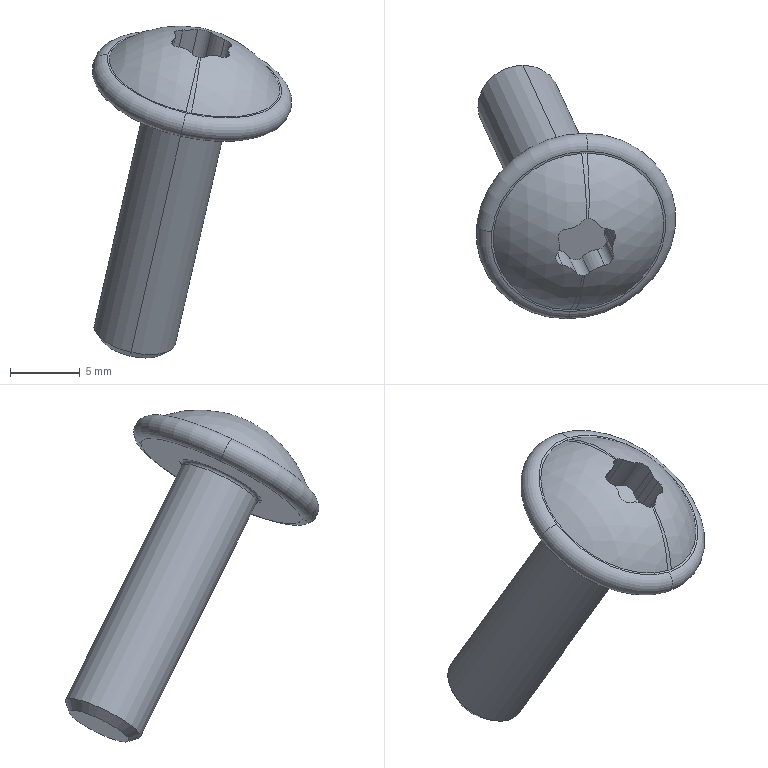Part | SolidWorks | features BaseBody 1 | 1 solid | 32 faces | box 14.289 x 18.177 x 23.78 mm | volume 994.304 mm3 | cylinder 17 | torus 5 | sphere 4 | plane 4 | cone 2 | commonest cylinder face diameters 1.32 x6 3.14 x4 2.34 x3 1.26 x2 6 x2
STEP:
#1=CARTESIAN_POINT('',(1919.161,-253.575,949.426));
#2=VERTEX_POINT('',#1);
#3=CARTESIAN_POINT('',(1919.214,-254.009,949.147));
#4=VERTEX_POINT('',#3);
#5=CARTESIAN_POINT('',(1919.161,-253.575,949.426));
#6=CARTESIAN_POINT('',(1919.144,-253.731,949.352));
#7=CARTESIAN_POINT('',(1919.162,-253.881,949.256));
#8=CARTESIAN_POINT('',(1919.214,-254.009,949.147));
#9=B_SPLINE_CURVE_WITH_KNOTS('',3,(#5,#6,#7,#8),.UNSPECIFIED.,.F.,.F.,(4,4),(0.000521,0.001041),.UNSPECIFIED.);
#10=EDGE_CURVE('',#2,#4,#9,.T.);
#11=ORIENTED_EDGE('',*,*,#10,.F.);
#12=CARTESIAN_POINT('',(1918.622,-252.41,947.083));
#13=VERTEX_POINT('',#12);
#14=CARTESIAN_POINT('',(1919.185,-253.627,949.532));
#15=DIRECTION('',(-0.2015,0.436,-0.8771));
#16=VECTOR('',#15,1000.);
#17=LINE('',#14,#16);
#18=EDGE_CURVE('',#2,#13,#17,.T.);
#19=ORIENTED_EDGE('',*,*,#18,.T.);
#20=CARTESIAN_POINT('',(1918.684,-252.864,946.843));
#21=VERTEX_POINT('',#20);
#22=CARTESIAN_POINT('',(1919.763,-252.41,946.821));
#23=DIRECTION('',(-0.2015,0.436,-0.8771));
#24=DIRECTION('',(-0.9216,-0.3877,0.01896));
#25=AXIS2_PLACEMENT_3D('',#22,#23,#24);
#26=CIRCLE('',#25,1.17);
#27=EDGE_CURVE('',#21,#13,#26,.T.);
#28=ORIENTED_EDGE('',*,*,#27,.F.);
#29=CARTESIAN_POINT('',(1918.684,-252.864,946.843));
#30=DIRECTION('',(0.2015,-0.436,0.8771));
#31=VECTOR('',#30,1000.);
#32=LINE('',#29,#31);
#33=EDGE_CURVE('',#21,#4,#32,.T.);
#34=ORIENTED_EDGE('',*,*,#33,.T.);
#35=EDGE_LOOP('',(#11,#19,#28,#34));
#36=FACE_OUTER_BOUND('',#35,.T.);
#37=CARTESIAN_POINT('',(1920.325,-253.627,949.27));
#38=DIRECTION('',(-0.2015,0.436,-0.8771));
#39=DIRECTION('',(-0.9746,0.,0.2239));
#40=AXIS2_PLACEMENT_3D('',#37,#38,#39);
#41=CYLINDRICAL_SURFACE('',#40,1.17);
#42=ADVANCED_FACE('',(#36),#41,.T.);
#43=CARTESIAN_POINT('',(1915.121,-254.247,949.922));
#44=VERTEX_POINT('',#43);
#45=CARTESIAN_POINT('',(1915.219,-254.009,950.064));
#46=VERTEX_POINT('',#45);
#47=CARTESIAN_POINT('',(1915.121,-254.247,949.922));
#48=CARTESIAN_POINT('',(1915.132,-254.163,949.973));
#49=CARTESIAN_POINT('',(1915.166,-254.081,950.021));
#50=CARTESIAN_POINT('',(1915.219,-254.009,950.064));
#51=B_SPLINE_CURVE_WITH_KNOTS('',3,(#47,#48,#49,#50),.UNSPECIFIED.,.F.,.F.,(4,4),(0.0009533,0.001248),.UNSPECIFIED.);
#52=EDGE_CURVE('',#44,#46,#51,.T.);
#53=ORIENTED_EDGE('',*,*,#52,.F.);
#54=CARTESIAN_POINT('',(1914.6,-253.12,947.654));
#55=VERTEX_POINT('',#54);
#56=CARTESIAN_POINT('',(1915.153,-254.317,950.064));
#57=DIRECTION('',(-0.2015,0.436,-0.8771));
#58=VECTOR('',#57,1000.);
#59=LINE('',#56,#58);
#60=EDGE_CURVE('',#44,#55,#59,.T.);
#61=ORIENTED_EDGE('',*,*,#60,.T.);
#62=CARTESIAN_POINT('',(1914.69,-252.864,947.761));
#63=VERTEX_POINT('',#62);
#64=CARTESIAN_POINT('',(1915.243,-253.12,947.506));
#65=DIRECTION('',(0.2015,-0.436,0.8771));
#66=DIRECTION('',(-0.8375,0.3877,0.3851));
#67=AXIS2_PLACEMENT_3D('',#64,#65,#66);
#68=CIRCLE('',#67,0.66);
#69=EDGE_CURVE('',#63,#55,#68,.T.);
#70=ORIENTED_EDGE('',*,*,#69,.F.);
#71=CARTESIAN_POINT('',(1914.69,-252.864,947.761));
#72=DIRECTION('',(0.2015,-0.436,0.8771));
#73=VECTOR('',#72,1000.);
#74=LINE('',#71,#73);
#75=EDGE_CURVE('',#63,#46,#74,.T.);
#76=ORIENTED_EDGE('',*,*,#75,.T.);
#77=EDGE_LOOP('',(#53,#61,#70,#76));
#78=FACE_OUTER_BOUND('',#77,.T.);
#79=CARTESIAN_POINT('',(1915.796,-254.317,949.916));
#80=DIRECTION('',(-0.2015,0.436,-0.8771));
#81=DIRECTION('',(-0.9746,0.,0.2239));
#82=AXIS2_PLACEMENT_3D('',#79,#80,#81);
#83=CYLINDRICAL_SURFACE('',#82,0.66);
#84=ADVANCED_FACE('',(#78),#83,.F.);
#85=CARTESIAN_POINT('',(1915.275,-252.828,950.593));
#86=VERTEX_POINT('',#85);
#87=CARTESIAN_POINT('',(1915.91,-252.257,950.777));
#88=VERTEX_POINT('',#87);
#89=CARTESIAN_POINT('',(1915.275,-252.828,950.593));
#90=CARTESIAN_POINT('',(1915.287,-252.679,950.646));
#91=CARTESIAN_POINT('',(1915.36,-252.533,950.696));
#92=CARTESIAN_POINT('',(1915.591,-252.325,950.763));
#93=CARTESIAN_POINT('',(1915.749,-252.263,950.781));
#94=CARTESIAN_POINT('',(1915.91,-252.257,950.777));
#95=B_SPLINE_CURVE_WITH_KNOTS('',3,(#89,#90,#91,#92,#93,#94),.UNSPECIFIED.,.F.,.F.,(4,2,4),(0.0002952,0.0007716,0.001248),.UNSPECIFIED.);
#96=EDGE_CURVE('',#86,#88,#95,.T.);
#97=ORIENTED_EDGE('',*,*,#96,.F.);
#98=CARTESIAN_POINT('',(1914.754,-251.701,948.324));
#99=VERTEX_POINT('',#98);
#100=CARTESIAN_POINT('',(1915.307,-252.898,950.734));
#101=DIRECTION('',(-0.2015,0.436,-0.8771));
#102=VECTOR('',#101,1000.);
#103=LINE('',#100,#102);
#104=EDGE_CURVE('',#86,#99,#103,.T.);
#105=ORIENTED_EDGE('',*,*,#104,.T.);
#106=CARTESIAN_POINT('',(1915.38,-251.111,948.473));
#107=VERTEX_POINT('',#106);
#108=CARTESIAN_POINT('',(1915.397,-251.701,948.177));
#109=DIRECTION('',(0.2015,-0.436,0.8771));
#110=DIRECTION('',(-0.0251,0.8929,0.4496));
#111=AXIS2_PLACEMENT_3D('',#108,#109,#110);
#112=CIRCLE('',#111,0.66);
#113=EDGE_CURVE('',#107,#99,#112,.T.);
#114=ORIENTED_EDGE('',*,*,#113,.F.);
#115=CARTESIAN_POINT('',(1915.38,-251.111,948.473));
#116=DIRECTION('',(0.2015,-0.436,0.8771));
#117=VECTOR('',#116,1000.);
#118=LINE('',#115,#117);
#119=EDGE_CURVE('',#107,#88,#118,.T.);
#120=ORIENTED_EDGE('',*,*,#119,.T.);
#121=EDGE_LOOP('',(#97,#105,#114,#120));
#122=FACE_OUTER_BOUND('',#121,.T.);
#123=CARTESIAN_POINT('',(1915.95,-252.898,950.586));
#124=DIRECTION('',(-0.2015,0.436,-0.8771));
#125=DIRECTION('',(-0.9746,0.,0.2239));
#126=AXIS2_PLACEMENT_3D('',#123,#124,#125);
#127=CYLINDRICAL_SURFACE('',#126,0.66);
#128=ADVANCED_FACE('',(#122),#127,.F.);
#129=CARTESIAN_POINT('',(1916.981,-251.727,950.799));
#130=VERTEX_POINT('',#129);
#131=CARTESIAN_POINT('',(1917.338,-251.504,950.774));
#132=VERTEX_POINT('',#131);
#133=CARTESIAN_POINT('',(1916.981,-251.727,950.799));
#134=CARTESIAN_POINT('',(1917.073,-251.616,950.806));
#135=CARTESIAN_POINT('',(1917.199,-251.537,950.798));
#136=CARTESIAN_POINT('',(1917.338,-251.504,950.774));
#137=B_SPLINE_CURVE_WITH_KNOTS('',3,(#133,#134,#135,#136),.UNSPECIFIED.,.F.,.F.,(4,4),(0.,0.0004276),.UNSPECIFIED.);
#138=EDGE_CURVE('',#130,#132,#137,.T.);
#139=ORIENTED_EDGE('',*,*,#138,.T.);
#140=CARTESIAN_POINT('',(1916.967,-246.837,950.279));
#141=VERTEX_POINT('',#140);
#142=CARTESIAN_POINT('',(1915.669,-250.1,942.87));
#143=DIRECTION('',(-0.9788,-0.05695,0.1965));
#144=DIRECTION('',(0.1968,0.,0.9804));
#145=AXIS2_PLACEMENT_3D('',#142,#143,#144);
#146=CIRCLE('',#145,8.2);
#147=EDGE_CURVE('',#132,#141,#146,.T.);
#148=ORIENTED_EDGE('',*,*,#147,.T.);
#149=CARTESIAN_POINT('',(1916.137,-258.03,944.906));
#150=VERTEX_POINT('',#149);
#151=CARTESIAN_POINT('',(1916.745,-252.427,947.551));
#152=DIRECTION('',(0.2015,-0.436,0.8771));
#153=DIRECTION('',(0.09761,0.8999,0.425));
#154=AXIS2_PLACEMENT_3D('',#151,#152,#153);
#155=CIRCLE('',#154,6.225);
#156=EDGE_CURVE('',#141,#150,#155,.T.);
#157=ORIENTED_EDGE('',*,*,#156,.T.);
#158=CARTESIAN_POINT('',(1917.034,-255.583,948.813));
#159=VERTEX_POINT('',#158);
#160=CARTESIAN_POINT('',(1915.669,-250.1,942.87));
#161=DIRECTION('',(-0.9746,0.,0.2239));
#162=DIRECTION('',(0.05704,-0.967,0.2483));
#163=AXIS2_PLACEMENT_3D('',#160,#161,#162);
#164=CIRCLE('',#163,8.2);
#165=EDGE_CURVE('',#150,#159,#164,.T.);
#166=ORIENTED_EDGE('',*,*,#165,.T.);
#167=CARTESIAN_POINT('',(1916.585,-255.387,949.071));
#168=VERTEX_POINT('',#167);
#169=CARTESIAN_POINT('',(1917.034,-255.583,948.813));
#170=CARTESIAN_POINT('',(1916.846,-255.583,948.856));
#171=CARTESIAN_POINT('',(1916.678,-255.508,948.953));
#172=CARTESIAN_POINT('',(1916.585,-255.387,949.071));
#173=B_SPLINE_CURVE_WITH_KNOTS('',3,(#169,#170,#171,#172),.UNSPECIFIED.,.F.,.F.,(4,4),(0.,0.0005707),.UNSPECIFIED.);
#174=EDGE_CURVE('',#159,#168,#173,.T.);
#175=ORIENTED_EDGE('',*,*,#174,.T.);
#176=CARTESIAN_POINT('',(1915.628,-254.854,949.551));
#177=VERTEX_POINT('',#176);
#178=CARTESIAN_POINT('',(1916.585,-255.387,949.071));
#179=CARTESIAN_POINT('',(1916.534,-255.322,949.134));
#180=CARTESIAN_POINT('',(1916.476,-255.261,949.191));
#181=CARTESIAN_POINT('',(1916.342,-255.149,949.297));
#182=CARTESIAN_POINT('',(1916.266,-255.096,949.345));
#183=CARTESIAN_POINT('',(1916.02,-254.959,949.469));
#184=CARTESIAN_POINT('',(1915.83,-254.892,949.525));
#185=CARTESIAN_POINT('',(1915.628,-254.854,949.551));
#186=B_SPLINE_CURVE_WITH_KNOTS('',3,(#178,#179,#180,#181,#182,#183,#184,#185),.UNSPECIFIED.,.F.,.F.,(4,2,2,4),(0.,0.0003062,0.0006125,0.001225),.UNSPECIFIED.);
#187=EDGE_CURVE('',#168,#177,#186,.T.);
#188=ORIENTED_EDGE('',*,*,#187,.T.);
#189=CARTESIAN_POINT('',(1915.628,-254.854,949.551));
#190=CARTESIAN_POINT('',(1915.471,-254.825,949.571));
#191=CARTESIAN_POINT('',(1915.33,-254.746,949.62));
#192=CARTESIAN_POINT('',(1915.144,-254.524,949.756));
#193=CARTESIAN_POINT('',(1915.102,-254.383,949.841));
#194=CARTESIAN_POINT('',(1915.121,-254.247,949.922));
#195=B_SPLINE_CURVE_WITH_KNOTS('',3,(#189,#190,#191,#192,#193,#194),.UNSPECIFIED.,.F.,.F.,(4,2,4),(0.,0.0004766,0.0009533),.UNSPECIFIED.);
#196=EDGE_CURVE('',#177,#44,#195,.T.);
#197=ORIENTED_EDGE('',*,*,#196,.T.);
#198=ORIENTED_EDGE('',*,*,#52,.T.);
#199=CARTESIAN_POINT('',(1915.318,-253.102,950.493));
#200=VERTEX_POINT('',#199);
#201=CARTESIAN_POINT('',(1915.219,-254.009,950.064));
#202=CARTESIAN_POINT('',(1915.266,-253.945,950.102));
#203=CARTESIAN_POINT('',(1915.304,-253.876,950.14));
#204=CARTESIAN_POINT('',(1915.361,-253.731,950.216));
#205=CARTESIAN_POINT('',(1915.38,-253.653,950.255));
#206=CARTESIAN_POINT('',(1915.406,-253.419,950.366));
#207=CARTESIAN_POINT('',(1915.381,-253.255,950.435));
#208=CARTESIAN_POINT('',(1915.318,-253.102,950.493));
#209=B_SPLINE_CURVE_WITH_KNOTS('',3,(#201,#202,#203,#204,#205,#206,#207,#208),.UNSPECIFIED.,.F.,.F.,(4,2,2,4),(0.,0.0002604,0.0005207,0.001041),.UNSPECIFIED.);
#210=EDGE_CURVE('',#46,#200,#209,.T.);
#211=ORIENTED_EDGE('',*,*,#210,.T.);
#212=CARTESIAN_POINT('',(1915.318,-253.102,950.493));
#213=CARTESIAN_POINT('',(1915.282,-253.014,950.525));
#214=CARTESIAN_POINT('',(1915.267,-252.921,950.559));
#215=CARTESIAN_POINT('',(1915.275,-252.828,950.593));
#216=B_SPLINE_CURVE_WITH_KNOTS('',3,(#212,#213,#214,#215),.UNSPECIFIED.,.F.,.F.,(4,4),(0.,0.0002952),.UNSPECIFIED.);
#217=EDGE_CURVE('',#200,#86,#216,.T.);
#218=ORIENTED_EDGE('',*,*,#217,.T.);
#219=ORIENTED_EDGE('',*,*,#96,.T.);
#220=CARTESIAN_POINT('',(1915.91,-252.257,950.777));
#221=CARTESIAN_POINT('',(1916.013,-252.253,950.775));
#222=CARTESIAN_POINT('',(1916.114,-252.238,950.774));
#223=CARTESIAN_POINT('',(1916.312,-252.189,950.774));
#224=CARTESIAN_POINT('',(1916.41,-252.153,950.775));
#225=CARTESIAN_POINT('',(1916.686,-252.017,950.78));
#226=CARTESIAN_POINT('',(1916.85,-251.887,950.788));
#227=CARTESIAN_POINT('',(1916.981,-251.727,950.799));
#228=B_SPLINE_CURVE_WITH_KNOTS('',3,(#220,#221,#222,#223,#224,#225,#226,#227),.UNSPECIFIED.,.F.,.F.,(4,2,2,4),(0.,0.0003062,0.0006125,0.001225),.UNSPECIFIED.);
#229=EDGE_CURVE('',#88,#130,#228,.T.);
#230=ORIENTED_EDGE('',*,*,#229,.T.);
#231=EDGE_LOOP('',(#139,#148,#157,#166,#175,#188,#197,#198,#211,#218,#219,#230));
#232=FACE_OUTER_BOUND('',#231,.T.);
#233=CARTESIAN_POINT('',(1915.669,-250.1,942.87));
#234=DIRECTION('',(-0.9788,-0.05695,0.1965));
#235=DIRECTION('',(-0.03574,-0.8981,-0.4383));
#236=AXIS2_PLACEMENT_3D('',#233,#234,#235);
#237=SPHERICAL_SURFACE('',#236,8.2);
#238=ADVANCED_FACE('',(#232),#237,.T.);
#239=CARTESIAN_POINT('',(1917.552,-255.387,948.849));
#240=VERTEX_POINT('',#239);
#241=CARTESIAN_POINT('',(1917.176,-255.569,948.791));
#242=VERTEX_POINT('',#241);
#243=CARTESIAN_POINT('',(1917.552,-255.387,948.849));
#244=CARTESIAN_POINT('',(1917.45,-255.478,948.8));
#245=CARTESIAN_POINT('',(1917.318,-255.543,948.779));
#246=CARTESIAN_POINT('',(1917.176,-255.569,948.791));
#247=B_SPLINE_CURVE_WITH_KNOTS('',3,(#243,#244,#245,#246),.UNSPECIFIED.,.F.,.F.,(4,4),(0.,0.0004276),.UNSPECIFIED.);
#248=EDGE_CURVE('',#240,#242,#247,.T.);
#249=ORIENTED_EDGE('',*,*,#248,.T.);
#250=CARTESIAN_POINT('',(1916.522,-258.018,944.823));
#251=VERTEX_POINT('',#250);
#252=CARTESIAN_POINT('',(1915.669,-250.1,942.87));
#253=DIRECTION('',(0.9788,0.05695,-0.1965));
#254=DIRECTION('',(-0.1968,0.,-0.9804));
#255=AXIS2_PLACEMENT_3D('',#252,#253,#254);
#256=CIRCLE('',#255,8.2);
#257=EDGE_CURVE('',#242,#251,#256,.T.);
#258=ORIENTED_EDGE('',*,*,#257,.T.);
#259=CARTESIAN_POINT('',(1917.352,-246.825,950.197));
#260=VERTEX_POINT('',#259);
#261=CARTESIAN_POINT('',(1916.745,-252.427,947.551));
#262=DIRECTION('',(-0.2015,0.436,-0.8771));
#263=DIRECTION('',(0.09761,0.8999,0.425));
#264=AXIS2_PLACEMENT_3D('',#261,#262,#263);
#265=CIRCLE('',#264,6.225);
#266=EDGE_CURVE('',#260,#251,#265,.T.);
#267=ORIENTED_EDGE('',*,*,#266,.F.);
#268=CARTESIAN_POINT('',(1917.478,-251.488,950.746));
#269=VERTEX_POINT('',#268);
#270=CARTESIAN_POINT('',(1915.669,-250.1,942.87));
#271=DIRECTION('',(-0.9746,0.,0.2239));
#272=DIRECTION('',(0.2052,0.3994,0.8935));
#273=AXIS2_PLACEMENT_3D('',#270,#271,#272);
#274=CIRCLE('',#273,8.2);
#275=EDGE_CURVE('',#269,#260,#274,.T.);
#276=ORIENTED_EDGE('',*,*,#275,.F.);
#277=CARTESIAN_POINT('',(1917.949,-251.727,950.577));
#278=VERTEX_POINT('',#277);
#279=CARTESIAN_POINT('',(1917.478,-251.488,950.746));
#280=CARTESIAN_POINT('',(1917.667,-251.488,950.703));
#281=CARTESIAN_POINT('',(1917.843,-251.579,950.639));
#282=CARTESIAN_POINT('',(1917.949,-251.727,950.577));
#283=B_SPLINE_CURVE_WITH_KNOTS('',3,(#279,#280,#281,#282),.UNSPECIFIED.,.F.,.F.,(4,4),(0.,0.0005707),.UNSPECIFIED.);
#284=EDGE_CURVE('',#269,#278,#283,.T.);
#285=ORIENTED_EDGE('',*,*,#284,.T.);
#286=CARTESIAN_POINT('',(1918.904,-252.257,950.09));
#287=VERTEX_POINT('',#286);
#288=CARTESIAN_POINT('',(1917.949,-251.727,950.577));
#289=CARTESIAN_POINT('',(1918.005,-251.807,950.543));
#290=CARTESIAN_POINT('',(1918.069,-251.879,950.507));
#291=CARTESIAN_POINT('',(1918.21,-252.006,950.43));
#292=CARTESIAN_POINT('',(1918.288,-252.062,950.389));
#293=CARTESIAN_POINT('',(1918.533,-252.198,950.264));
#294=CARTESIAN_POINT('',(1918.716,-252.249,950.176));
#295=CARTESIAN_POINT('',(1918.904,-252.257,950.09));
#296=B_SPLINE_CURVE_WITH_KNOTS('',3,(#288,#289,#290,#291,#292,#293,#294,#295),.UNSPECIFIED.,.F.,.F.,(4,2,2,4),(0.,0.0003062,0.0006125,0.001225),.UNSPECIFIED.);
#297=EDGE_CURVE('',#278,#287,#296,.T.);
#298=ORIENTED_EDGE('',*,*,#297,.T.);
#299=CARTESIAN_POINT('',(1919.312,-253.102,949.575));
#300=VERTEX_POINT('',#299);
#301=CARTESIAN_POINT('',(1918.904,-252.257,950.09));
#302=CARTESIAN_POINT('',(1918.999,-252.261,950.046));
#303=CARTESIAN_POINT('',(1919.089,-252.288,949.995));
#304=CARTESIAN_POINT('',(1919.241,-252.384,949.889));
#305=CARTESIAN_POINT('',(1919.303,-252.453,949.835));
#306=CARTESIAN_POINT('',(1919.383,-252.618,949.734));
#307=CARTESIAN_POINT('',(1919.401,-252.714,949.688));
#308=CARTESIAN_POINT('',(1919.39,-252.91,949.616));
#309=CARTESIAN_POINT('',(1919.361,-253.009,949.59));
#310=CARTESIAN_POINT('',(1919.312,-253.102,949.575));
#311=B_SPLINE_CURVE_WITH_KNOTS('',3,(#301,#302,#303,#304,#305,#306,#307,#308,#309,#310),.UNSPECIFIED.,.F.,.F.,(4,2,2,2,4),(0.,0.000312,0.000624,0.0009359,0.001248),.UNSPECIFIED.);
#312=EDGE_CURVE('',#287,#300,#311,.T.);
#313=ORIENTED_EDGE('',*,*,#312,.T.);
#314=CARTESIAN_POINT('',(1919.312,-253.102,949.575));
#315=CARTESIAN_POINT('',(1919.271,-253.178,949.563));
#316=CARTESIAN_POINT('',(1919.237,-253.257,949.544));
#317=CARTESIAN_POINT('',(1919.186,-253.415,949.494));
#318=CARTESIAN_POINT('',(1919.169,-253.496,949.462));
#319=CARTESIAN_POINT('',(1919.161,-253.575,949.426));
#320=B_SPLINE_CURVE_WITH_KNOTS('',3,(#314,#315,#316,#317,#318,#319),.UNSPECIFIED.,.F.,.F.,(4,2,4),(0.,0.0002605,0.000521),.UNSPECIFIED.);
#321=EDGE_CURVE('',#300,#2,#320,.T.);
#322=ORIENTED_EDGE('',*,*,#321,.T.);
#323=ORIENTED_EDGE('',*,*,#10,.T.);
#324=CARTESIAN_POINT('',(1918.622,-254.854,948.863));
#325=VERTEX_POINT('',#324);
#326=CARTESIAN_POINT('',(1919.214,-254.009,949.147));
#327=CARTESIAN_POINT('',(1919.245,-254.086,949.081));
#328=CARTESIAN_POINT('',(1919.253,-254.173,949.02));
#329=CARTESIAN_POINT('',(1919.224,-254.35,948.916));
#330=CARTESIAN_POINT('',(1919.186,-254.441,948.873));
#331=CARTESIAN_POINT('',(1919.07,-254.607,948.818));
#332=CARTESIAN_POINT('',(1918.993,-254.681,948.805));
#333=CARTESIAN_POINT('',(1918.818,-254.795,948.811));
#334=CARTESIAN_POINT('',(1918.72,-254.835,948.83));
#335=CARTESIAN_POINT('',(1918.622,-254.854,948.863));
#336=B_SPLINE_CURVE_WITH_KNOTS('',3,(#326,#327,#328,#329,#330,#331,#332,#333,#334,#335),.UNSPECIFIED.,.F.,.F.,(4,2,2,2,4),(0.,0.000312,0.000624,0.000936,0.001248),.UNSPECIFIED.);
#337=EDGE_CURVE('',#4,#325,#336,.T.);
#338=ORIENTED_EDGE('',*,*,#337,.T.);
#339=CARTESIAN_POINT('',(1918.622,-254.854,948.863));
#340=CARTESIAN_POINT('',(1918.526,-254.873,948.895));
#341=CARTESIAN_POINT('',(1918.43,-254.899,948.92));
#342=CARTESIAN_POINT('',(1918.239,-254.964,948.951));
#343=CARTESIAN_POINT('',(1918.143,-255.005,948.959));
#344=CARTESIAN_POINT('',(1917.867,-255.141,948.955));
#345=CARTESIAN_POINT('',(1917.697,-255.257,948.918));
#346=CARTESIAN_POINT('',(1917.552,-255.387,948.849));
#347=B_SPLINE_CURVE_WITH_KNOTS('',3,(#339,#340,#341,#342,#343,#344,#345,#346),.UNSPECIFIED.,.F.,.F.,(4,2,2,4),(0.,0.0003062,0.0006125,0.001225),.UNSPECIFIED.);
#348=EDGE_CURVE('',#325,#240,#347,.T.);
#349=ORIENTED_EDGE('',*,*,#348,.T.);
#350=EDGE_LOOP('',(#249,#258,#267,#276,#285,#298,#313,#322,#323,#338,#349));
#351=FACE_OUTER_BOUND('',#350,.T.);
#352=CARTESIAN_POINT('',(1915.669,-250.1,942.87));
#353=DIRECTION('',(0.9788,0.05695,-0.1965));
#354=DIRECTION('',(0.03574,0.8981,0.4383));
#355=AXIS2_PLACEMENT_3D('',#352,#353,#354);
#356=SPHERICAL_SURFACE('',#355,8.2);
#357=ADVANCED_FACE('',(#351),#356,.T.);
#358=CARTESIAN_POINT('',(1910.531,-252.427,948.978));
#359=VERTEX_POINT('',#358);
#360=CARTESIAN_POINT('',(1916.122,-258.165,944.842));
#361=VERTEX_POINT('',#360);
#362=CARTESIAN_POINT('',(1916.745,-252.427,947.551));
#363=DIRECTION('',(0.2015,-0.436,0.8771));
#364=DIRECTION('',(0.09761,0.8999,0.425));
#365=AXIS2_PLACEMENT_3D('',#362,#363,#364);
#366=CIRCLE('',#365,6.375);
#367=EDGE_CURVE('',#359,#361,#366,.T.);
#368=ORIENTED_EDGE('',*,*,#367,.F.);
#369=CARTESIAN_POINT('',(1910.169,-251.643,947.4));
#370=VERTEX_POINT('',#369);
#371=CARTESIAN_POINT('',(1910.35,-252.035,948.189));
#372=DIRECTION('',(-0.09761,-0.8999,-0.425));
#373=DIRECTION('',(0.,0.427,-0.9043));
#374=AXIS2_PLACEMENT_3D('',#371,#372,#373);
#375=CIRCLE('',#374,0.9);
#376=EDGE_CURVE('',#359,#370,#375,.T.);
#377=ORIENTED_EDGE('',*,*,#376,.T.);
#378=CARTESIAN_POINT('',(1915.76,-257.38,943.263));
#379=VERTEX_POINT('',#378);
#380=CARTESIAN_POINT('',(1916.382,-251.643,945.972));
#381=DIRECTION('',(0.2015,-0.436,0.8771));
#382=DIRECTION('',(0.09761,0.8999,0.425));
#383=AXIS2_PLACEMENT_3D('',#380,#381,#382);
#384=CIRCLE('',#383,6.375);
#385=EDGE_CURVE('',#370,#379,#384,.T.);
#386=ORIENTED_EDGE('',*,*,#385,.T.);
#387=CARTESIAN_POINT('',(1915.941,-257.772,944.053));
#388=DIRECTION('',(0.9746,0.,-0.2239));
#389=DIRECTION('',(-0.2015,0.436,-0.8771));
#390=AXIS2_PLACEMENT_3D('',#387,#388,#389);
#391=CIRCLE('',#390,0.9);
#392=EDGE_CURVE('',#361,#379,#391,.T.);
#393=ORIENTED_EDGE('',*,*,#392,.F.);
#394=EDGE_LOOP('',(#368,#377,#386,#393));
#395=FACE_OUTER_BOUND('',#394,.T.);
#396=CARTESIAN_POINT('',(1916.563,-252.035,946.762));
#397=DIRECTION('',(-0.2015,0.436,-0.8771));
#398=DIRECTION('',(-0.9746,0.,0.2239));
#399=AXIS2_PLACEMENT_3D('',#396,#397,#398);
#400=TOROIDAL_SURFACE('',#399,6.375,0.9);
#401=ADVANCED_FACE('',(#395),#400,.T.);
#402=CARTESIAN_POINT('',(1912.584,-240.785,929.44));
#403=VERTEX_POINT('',#402);
#404=CARTESIAN_POINT('',(1912.121,-245.06,927.421));
#405=VERTEX_POINT('',#404);
#406=CARTESIAN_POINT('',(1912.353,-242.922,928.43));
#407=DIRECTION('',(-0.2015,0.436,-0.8771));
#408=DIRECTION('',(0.09761,0.8999,0.425));
#409=AXIS2_PLACEMENT_3D('',#406,#407,#408);
#410=CIRCLE('',#409,2.375);
#411=EDGE_CURVE('',#403,#405,#410,.T.);
#412=ORIENTED_EDGE('',*,*,#411,.T.);
#413=CARTESIAN_POINT('',(1912.353,-242.922,928.43));
#414=DIRECTION('',(-0.2015,0.436,-0.8771));
#415=DIRECTION('',(-0.09761,-0.8999,-0.425));
#416=AXIS2_PLACEMENT_3D('',#413,#414,#415);
#417=CIRCLE('',#416,2.375);
#418=EDGE_CURVE('',#405,#403,#417,.T.);
#419=ORIENTED_EDGE('',*,*,#418,.T.);
#420=EDGE_LOOP('',(#412,#419));
#421=FACE_OUTER_BOUND('',#420,.T.);
#422=CARTESIAN_POINT('',(1915.042,-240.677,928.929));
#423=DIRECTION('',(-0.2015,0.436,-0.8771));
#424=DIRECTION('',(-0.09761,-0.8999,-0.425));
#425=AXIS2_PLACEMENT_3D('',#422,#423,#424);
#426=PLANE('',#425);
#427=ADVANCED_FACE('',(#421),#426,.T.);
#428=CARTESIAN_POINT('',(1912.186,-245.895,927.704));
#429=VERTEX_POINT('',#428);
#430=CARTESIAN_POINT('',(1912.121,-245.06,927.421));
#431=DIRECTION('',(-0.07344,0.9447,-0.3197));
#432=VECTOR('',#431,1000.);
#433=LINE('',#430,#432);
#434=EDGE_CURVE('',#429,#405,#433,.T.);
#435=ORIENTED_EDGE('',*,*,#434,.F.);
#436=CARTESIAN_POINT('',(1912.771,-240.495,930.253));
#437=VERTEX_POINT('',#436);
#438=CARTESIAN_POINT('',(1912.479,-243.195,928.979));
#439=DIRECTION('',(-0.2015,0.436,-0.8771));
#440=DIRECTION('',(-0.09761,-0.8999,-0.425));
#441=AXIS2_PLACEMENT_3D('',#438,#439,#440);
#442=CIRCLE('',#441,3.);
#443=EDGE_CURVE('',#429,#437,#442,.T.);
#444=ORIENTED_EDGE('',*,*,#443,.T.);
#445=CARTESIAN_POINT('',(1912.584,-240.785,929.44));
#446=DIRECTION('',(0.2115,0.328,0.9207));
#447=VECTOR('',#446,1000.);
#448=LINE('',#445,#447);
#449=EDGE_CURVE('',#403,#437,#448,.T.);
#450=ORIENTED_EDGE('',*,*,#449,.F.);
#451=ORIENTED_EDGE('',*,*,#418,.F.);
#452=EDGE_LOOP('',(#435,#444,#450,#451));
#453=FACE_OUTER_BOUND('',#452,.T.);
#454=CARTESIAN_POINT('',(1912.496,-243.232,929.053));
#455=DIRECTION('',(0.2015,-0.436,0.8771));
#456=DIRECTION('',(-0.09761,-0.8999,-0.425));
#457=AXIS2_PLACEMENT_3D('',#454,#455,#456);
#458=CONICAL_SURFACE('',#457,3.085,0.7854);
#459=ADVANCED_FACE('',(#453),#458,.T.);
#460=ORIENTED_EDGE('',*,*,#449,.T.);
#461=CARTESIAN_POINT('',(1912.479,-243.195,928.979));
#462=DIRECTION('',(-0.2015,0.436,-0.8771));
#463=DIRECTION('',(0.09761,0.8999,0.425));
#464=AXIS2_PLACEMENT_3D('',#461,#462,#463);
#465=CIRCLE('',#464,3.);
#466=EDGE_CURVE('',#437,#429,#465,.T.);
#467=ORIENTED_EDGE('',*,*,#466,.T.);
#468=ORIENTED_EDGE('',*,*,#434,.T.);
#469=ORIENTED_EDGE('',*,*,#411,.F.);
#470=EDGE_LOOP('',(#460,#467,#468,#469));
#471=FACE_OUTER_BOUND('',#470,.T.);
#472=CARTESIAN_POINT('',(1912.496,-243.232,929.053));
#473=DIRECTION('',(0.2015,-0.436,0.8771));
#474=DIRECTION('',(-0.09761,-0.8999,-0.425));
#475=AXIS2_PLACEMENT_3D('',#472,#473,#474);
#476=CONICAL_SURFACE('',#475,3.085,0.7854);
#477=ADVANCED_FACE('',(#471),#476,.T.);
#478=CARTESIAN_POINT('',(1916.039,-254.233,944.478));
#479=VERTEX_POINT('',#478);
#480=CARTESIAN_POINT('',(1916.039,-254.233,944.478));
#481=DIRECTION('',(-0.2015,0.436,-0.8771));
#482=VECTOR('',#481,1000.);
#483=LINE('',#480,#482);
#484=EDGE_CURVE('',#479,#429,#483,.T.);
#485=ORIENTED_EDGE('',*,*,#484,.T.);
#486=ORIENTED_EDGE('',*,*,#466,.F.);
#487=CARTESIAN_POINT('',(1916.624,-248.834,947.028));
#488=VERTEX_POINT('',#487);
#489=CARTESIAN_POINT('',(1916.624,-248.834,947.028));
#490=DIRECTION('',(0.2015,-0.436,0.8771));
#491=VECTOR('',#490,1000.);
#492=LINE('',#489,#491);
#493=EDGE_CURVE('',#437,#488,#492,.T.);
#494=ORIENTED_EDGE('',*,*,#493,.T.);
#495=CARTESIAN_POINT('',(1916.332,-251.534,945.753));
#496=DIRECTION('',(-0.2015,0.436,-0.8771));
#497=DIRECTION('',(0.09761,0.8999,0.425));
#498=AXIS2_PLACEMENT_3D('',#495,#496,#497);
#499=CIRCLE('',#498,3.);
#500=EDGE_CURVE('',#488,#479,#499,.T.);
#501=ORIENTED_EDGE('',*,*,#500,.T.);
#502=EDGE_LOOP('',(#485,#486,#494,#501));
#503=FACE_OUTER_BOUND('',#502,.T.);
#504=CARTESIAN_POINT('',(1916.409,-251.7,946.089));
#505=DIRECTION('',(-0.2015,0.436,-0.8771));
#506=DIRECTION('',(0.09761,0.8999,0.425));
#507=AXIS2_PLACEMENT_3D('',#504,#505,#506);
#508=CYLINDRICAL_SURFACE('',#507,3.);
#509=ADVANCED_FACE('',(#503),#508,.T.);
#510=CARTESIAN_POINT('',(1916.065,-254.567,944.591));
#511=VERTEX_POINT('',#510);
#512=CARTESIAN_POINT('',(1916.014,-254.458,944.372));
#513=DIRECTION('',(0.9746,0.,-0.2239));
#514=DIRECTION('',(0.2015,-0.436,0.8771));
#515=AXIS2_PLACEMENT_3D('',#512,#513,#514);
#516=CIRCLE('',#515,0.25);
#517=EDGE_CURVE('',#479,#511,#516,.T.);
#518=ORIENTED_EDGE('',*,*,#517,.F.);
#519=ORIENTED_EDGE('',*,*,#500,.F.);
#520=CARTESIAN_POINT('',(1916.699,-248.718,947.354));
#521=VERTEX_POINT('',#520);
#522=CARTESIAN_POINT('',(1916.649,-248.609,947.134));
#523=DIRECTION('',(0.9746,0.,-0.2239));
#524=DIRECTION('',(0.2015,-0.436,0.8771));
#525=AXIS2_PLACEMENT_3D('',#522,#523,#524);
#526=CIRCLE('',#525,0.25);
#527=EDGE_CURVE('',#521,#488,#526,.T.);
#528=ORIENTED_EDGE('',*,*,#527,.F.);
#529=CARTESIAN_POINT('',(1916.382,-251.643,945.972));
#530=DIRECTION('',(-0.2015,0.436,-0.8771));
#531=DIRECTION('',(0.09761,0.8999,0.425));
#532=AXIS2_PLACEMENT_3D('',#529,#530,#531);
#533=CIRCLE('',#532,3.25);
#534=EDGE_CURVE('',#521,#511,#533,.T.);
#535=ORIENTED_EDGE('',*,*,#534,.T.);
#536=EDGE_LOOP('',(#518,#519,#528,#535));
#537=FACE_OUTER_BOUND('',#536,.T.);
#538=CARTESIAN_POINT('',(1916.332,-251.534,945.753));
#539=DIRECTION('',(-0.2015,0.436,-0.8771));
#540=DIRECTION('',(0.09761,0.8999,0.425));
#541=AXIS2_PLACEMENT_3D('',#538,#539,#540);
#542=TOROIDAL_SURFACE('',#541,3.25,0.25);
#543=ADVANCED_FACE('',(#537),#542,.F.);
#544=CARTESIAN_POINT('',(1917.004,-245.906,948.681));
#545=VERTEX_POINT('',#544);
#546=CARTESIAN_POINT('',(1916.382,-251.643,945.972));
#547=DIRECTION('',(0.2015,-0.436,0.8771));
#548=DIRECTION('',(0.09761,0.8999,0.425));
#549=AXIS2_PLACEMENT_3D('',#546,#547,#548);
#550=CIRCLE('',#549,6.375);
#551=EDGE_CURVE('',#545,#370,#550,.T.);
#552=ORIENTED_EDGE('',*,*,#551,.F.);
#553=CARTESIAN_POINT('',(1916.382,-251.643,945.972));
#554=DIRECTION('',(-0.2015,0.436,-0.8771));
#555=DIRECTION('',(0.09761,0.8999,0.425));
#556=AXIS2_PLACEMENT_3D('',#553,#554,#555);
#557=CIRCLE('',#556,6.375);
#558=EDGE_CURVE('',#545,#379,#557,.T.);
#559=ORIENTED_EDGE('',*,*,#558,.T.);
#560=ORIENTED_EDGE('',*,*,#385,.F.);
#561=EDGE_LOOP('',(#552,#559,#560));
#562=FACE_OUTER_BOUND('',#561,.T.);
#563=CARTESIAN_POINT('',(1916.382,-251.643,945.972));
#564=DIRECTION('',(-0.2015,0.436,-0.8771));
#565=DIRECTION('',(-0.09761,-0.8999,-0.425));
#566=AXIS2_PLACEMENT_3D('',#563,#564,#565);
#567=CIRCLE('',#566,3.25);
#568=EDGE_CURVE('',#511,#521,#567,.T.);
#569=ORIENTED_EDGE('',*,*,#568,.F.);
#570=ORIENTED_EDGE('',*,*,#534,.F.);
#571=EDGE_LOOP('',(#569,#570));
#572=FACE_BOUND('',#571,.T.);
#573=CARTESIAN_POINT('',(1923.491,-245.676,947.306));
#574=DIRECTION('',(-0.2015,0.436,-0.8771));
#575=DIRECTION('',(-0.09761,-0.8999,-0.425));
#576=AXIS2_PLACEMENT_3D('',#573,#574,#575);
#577=PLANE('',#576);
#578=ADVANCED_FACE('',(#562,#572),#577,.T.);
#579=CARTESIAN_POINT('',(1917.367,-246.69,950.26));
#580=VERTEX_POINT('',#579);
#581=CARTESIAN_POINT('',(1916.745,-252.427,947.551));
#582=DIRECTION('',(-0.2015,0.436,-0.8771));
#583=DIRECTION('',(0.09761,0.8999,0.425));
#584=AXIS2_PLACEMENT_3D('',#581,#582,#583);
#585=CIRCLE('',#584,6.375);
#586=EDGE_CURVE('',#580,#361,#585,.T.);
#587=ORIENTED_EDGE('',*,*,#586,.T.);
#588=ORIENTED_EDGE('',*,*,#392,.T.);
#589=ORIENTED_EDGE('',*,*,#558,.F.);
#590=CARTESIAN_POINT('',(1917.186,-246.298,949.471));
#591=DIRECTION('',(0.9746,0.,-0.2239));
#592=DIRECTION('',(-0.2015,0.436,-0.8771));
#593=AXIS2_PLACEMENT_3D('',#590,#591,#592);
#594=CIRCLE('',#593,0.9);
#595=EDGE_CURVE('',#545,#580,#594,.T.);
#596=ORIENTED_EDGE('',*,*,#595,.T.);
#597=EDGE_LOOP('',(#587,#588,#589,#596));
#598=FACE_OUTER_BOUND('',#597,.T.);
#599=CARTESIAN_POINT('',(1916.563,-252.035,946.762));
#600=DIRECTION('',(-0.2015,0.436,-0.8771));
#601=DIRECTION('',(-0.9746,0.,0.2239));
#602=AXIS2_PLACEMENT_3D('',#599,#600,#601);
#603=TOROIDAL_SURFACE('',#602,6.375,0.9);
#604=ADVANCED_FACE('',(#598),#603,.T.);
#605=ORIENTED_EDGE('',*,*,#376,.F.);
#606=CARTESIAN_POINT('',(1916.745,-252.427,947.551));
#607=DIRECTION('',(0.2015,-0.436,0.8771));
#608=DIRECTION('',(0.09761,0.8999,0.425));
#609=AXIS2_PLACEMENT_3D('',#606,#607,#608);
#610=CIRCLE('',#609,6.375);
#611=EDGE_CURVE('',#580,#359,#610,.T.);
#612=ORIENTED_EDGE('',*,*,#611,.F.);
#613=ORIENTED_EDGE('',*,*,#595,.F.);
#614=ORIENTED_EDGE('',*,*,#551,.T.);
#615=EDGE_LOOP('',(#605,#612,#613,#614));
#616=FACE_OUTER_BOUND('',#615,.T.);
#617=CARTESIAN_POINT('',(1916.563,-252.035,946.762));
#618=DIRECTION('',(-0.2015,0.436,-0.8771));
#619=DIRECTION('',(-0.9746,0.,0.2239));
#620=AXIS2_PLACEMENT_3D('',#617,#618,#619);
#621=TOROIDAL_SURFACE('',#620,6.375,0.9);
#622=ADVANCED_FACE('',(#616),#621,.T.);
#623=ORIENTED_EDGE('',*,*,#586,.F.);
#624=ORIENTED_EDGE('',*,*,#611,.T.);
#625=ORIENTED_EDGE('',*,*,#367,.T.);
#626=EDGE_LOOP('',(#623,#624,#625));
#627=FACE_OUTER_BOUND('',#626,.T.);
#628=CARTESIAN_POINT('',(1916.745,-252.427,947.551));
#629=DIRECTION('',(0.2015,-0.436,0.8771));
#630=DIRECTION('',(0.09761,0.8999,0.425));
#631=AXIS2_PLACEMENT_3D('',#628,#629,#630);
#632=CIRCLE('',#631,6.225);
#633=EDGE_CURVE('',#260,#141,#632,.T.);
#634=ORIENTED_EDGE('',*,*,#633,.F.);
#635=ORIENTED_EDGE('',*,*,#266,.T.);
#636=CARTESIAN_POINT('',(1916.745,-252.427,947.551));
#637=DIRECTION('',(-0.2015,0.436,-0.8771));
#638=DIRECTION('',(0.09761,0.8999,0.425));
#639=AXIS2_PLACEMENT_3D('',#636,#637,#638);
#640=CIRCLE('',#639,6.225);
#641=EDGE_CURVE('',#251,#150,#640,.T.);
#642=ORIENTED_EDGE('',*,*,#641,.T.);
#643=ORIENTED_EDGE('',*,*,#156,.F.);
#644=EDGE_LOOP('',(#634,#635,#642,#643));
#645=FACE_BOUND('',#644,.T.);
#646=CARTESIAN_POINT('',(1923.853,-246.461,948.884));
#647=DIRECTION('',(0.2015,-0.436,0.8771));
#648=DIRECTION('',(-0.9746,0.,0.2239));
#649=AXIS2_PLACEMENT_3D('',#646,#647,#648);
#650=PLANE('',#649);
#651=ADVANCED_FACE('',(#627,#645),#650,.T.);
#652=ORIENTED_EDGE('',*,*,#257,.F.);
#653=CARTESIAN_POINT('',(1917.176,-255.569,948.791));
#654=CARTESIAN_POINT('',(1917.129,-255.578,948.795));
#655=CARTESIAN_POINT('',(1917.082,-255.583,948.802));
#656=CARTESIAN_POINT('',(1917.034,-255.583,948.813));
#657=B_SPLINE_CURVE_WITH_KNOTS('',3,(#653,#654,#655,#656),.UNSPECIFIED.,.F.,.F.,(4,4),(0.0004276,0.0005708),.UNSPECIFIED.);
#658=EDGE_CURVE('',#242,#159,#657,.T.);
#659=ORIENTED_EDGE('',*,*,#658,.T.);
#660=ORIENTED_EDGE('',*,*,#165,.F.);
#661=ORIENTED_EDGE('',*,*,#641,.F.);
#662=EDGE_LOOP('',(#652,#659,#660,#661));
#663=FACE_OUTER_BOUND('',#662,.T.);
#664=CARTESIAN_POINT('',(1915.669,-250.1,942.87));
#665=DIRECTION('',(0.9788,0.05695,-0.1965));
#666=DIRECTION('',(0.03574,0.8981,0.4383));
#667=AXIS2_PLACEMENT_3D('',#664,#665,#666);
#668=SPHERICAL_SURFACE('',#667,8.2);
#669=ADVANCED_FACE('',(#663),#668,.T.);
#670=CARTESIAN_POINT('',(1916.055,-254.24,946.763));
#671=VERTEX_POINT('',#670);
#672=CARTESIAN_POINT('',(1917.022,-254.24,946.541));
#673=VERTEX_POINT('',#672);
#674=CARTESIAN_POINT('',(1916.576,-253.89,946.817));
#675=DIRECTION('',(0.2015,-0.436,0.8771));
#676=DIRECTION('',(-0.8277,-0.5546,-0.08559));
#677=AXIS2_PLACEMENT_3D('',#674,#675,#676);
#678=CIRCLE('',#677,0.63);
#679=EDGE_CURVE('',#671,#673,#678,.T.);
#680=ORIENTED_EDGE('',*,*,#679,.F.);
#681=CARTESIAN_POINT('',(1916.055,-254.24,946.763));
#682=DIRECTION('',(0.2015,-0.436,0.8771));
#683=VECTOR('',#682,1000.);
#684=LINE('',#681,#683);
#685=EDGE_CURVE('',#671,#168,#684,.T.);
#686=ORIENTED_EDGE('',*,*,#685,.T.);
#687=ORIENTED_EDGE('',*,*,#174,.F.);
#688=ORIENTED_EDGE('',*,*,#658,.F.);
#689=ORIENTED_EDGE('',*,*,#248,.F.);
#690=CARTESIAN_POINT('',(1917.022,-254.24,946.541));
#691=DIRECTION('',(0.2015,-0.436,0.8771));
#692=VECTOR('',#691,1000.);
#693=LINE('',#690,#692);
#694=EDGE_CURVE('',#673,#240,#693,.T.);
#695=ORIENTED_EDGE('',*,*,#694,.F.);
#696=EDGE_LOOP('',(#680,#686,#687,#688,#689,#695));
#697=FACE_OUTER_BOUND('',#696,.T.);
#698=CARTESIAN_POINT('',(1917.13,-255.09,949.23));
#699=DIRECTION('',(-0.2015,0.436,-0.8771));
#700=DIRECTION('',(-0.9746,0.,0.2239));
#701=AXIS2_PLACEMENT_3D('',#698,#699,#700);
#702=CYLINDRICAL_SURFACE('',#701,0.63);
#703=ADVANCED_FACE('',(#697),#702,.F.);
#704=ORIENTED_EDGE('',*,*,#348,.F.);
#705=CARTESIAN_POINT('',(1918.093,-253.709,946.559));
#706=VERTEX_POINT('',#705);
#707=CARTESIAN_POINT('',(1918.093,-253.709,946.559));
#708=DIRECTION('',(0.2015,-0.436,0.8771));
#709=VECTOR('',#708,1000.);
#710=LINE('',#707,#709);
#711=EDGE_CURVE('',#706,#325,#710,.T.);
#712=ORIENTED_EDGE('',*,*,#711,.F.);
#713=CARTESIAN_POINT('',(1918.132,-255.111,945.853));
#714=DIRECTION('',(-0.2015,0.436,-0.8771));
#715=DIRECTION('',(-0.7074,0.5546,0.4382));
#716=AXIS2_PLACEMENT_3D('',#713,#714,#715);
#717=CIRCLE('',#716,1.57);
#718=EDGE_CURVE('',#673,#706,#717,.T.);
#719=ORIENTED_EDGE('',*,*,#718,.F.);
#720=ORIENTED_EDGE('',*,*,#694,.T.);
#721=EDGE_LOOP('',(#704,#712,#719,#720));
#722=FACE_OUTER_BOUND('',#721,.T.);
#723=CARTESIAN_POINT('',(1918.696,-256.332,948.309));
#724=DIRECTION('',(-0.2015,0.436,-0.8771));
#725=DIRECTION('',(0.09761,0.8999,0.425));
#726=AXIS2_PLACEMENT_3D('',#723,#724,#725);
#727=CYLINDRICAL_SURFACE('',#726,1.57);
#728=ADVANCED_FACE('',(#722),#727,.T.);
#729=ORIENTED_EDGE('',*,*,#718,.T.);
#730=CARTESIAN_POINT('',(1918.076,-253.12,946.856));
#731=DIRECTION('',(0.2015,-0.436,0.8771));
#732=DIRECTION('',(0.0251,-0.8929,-0.4496));
#733=AXIS2_PLACEMENT_3D('',#730,#731,#732);
#734=CIRCLE('',#733,0.66);
#735=EDGE_CURVE('',#706,#21,#734,.T.);
#736=ORIENTED_EDGE('',*,*,#735,.T.);
#737=ORIENTED_EDGE('',*,*,#27,.T.);
#738=CARTESIAN_POINT('',(1918.783,-251.956,947.272));
#739=VERTEX_POINT('',#738);
#740=CARTESIAN_POINT('',(1919.763,-252.41,946.821));
#741=DIRECTION('',(-0.2015,0.436,-0.8771));
#742=DIRECTION('',(-0.9216,-0.3877,0.01896));
#743=AXIS2_PLACEMENT_3D('',#740,#741,#742);
#744=CIRCLE('',#743,1.17);
#745=EDGE_CURVE('',#13,#739,#744,.T.);
#746=ORIENTED_EDGE('',*,*,#745,.T.);
#747=CARTESIAN_POINT('',(1918.375,-251.111,947.786));
#748=VERTEX_POINT('',#747);
#749=CARTESIAN_POINT('',(1918.23,-251.701,947.526));
#750=DIRECTION('',(0.2015,-0.436,0.8771));
#751=DIRECTION('',(0.8375,-0.3877,-0.3851));
#752=AXIS2_PLACEMENT_3D('',#749,#750,#751);
#753=CIRCLE('',#752,0.66);
#754=EDGE_CURVE('',#739,#748,#753,.T.);
#755=ORIENTED_EDGE('',*,*,#754,.T.);
#756=CARTESIAN_POINT('',(1917.419,-250.58,948.269));
#757=VERTEX_POINT('',#756);
#758=CARTESIAN_POINT('',(1918.718,-249.709,948.403));
#759=DIRECTION('',(-0.2015,0.436,-0.8771));
#760=DIRECTION('',(-0.2188,-0.8929,-0.3936));
#761=AXIS2_PLACEMENT_3D('',#758,#759,#760);
#762=CIRCLE('',#761,1.57);
#763=EDGE_CURVE('',#748,#757,#762,.T.);
#764=ORIENTED_EDGE('',*,*,#763,.T.);
#765=CARTESIAN_POINT('',(1916.451,-250.58,948.491));
#766=VERTEX_POINT('',#765);
#767=CARTESIAN_POINT('',(1916.897,-250.93,948.215));
#768=DIRECTION('',(0.2015,-0.436,0.8771));
#769=DIRECTION('',(0.8277,0.5546,0.08559));
#770=AXIS2_PLACEMENT_3D('',#767,#768,#769);
#771=CIRCLE('',#770,0.63);
#772=EDGE_CURVE('',#757,#766,#771,.T.);
#773=ORIENTED_EDGE('',*,*,#772,.T.);
#774=CARTESIAN_POINT('',(1915.341,-249.709,949.179));
#775=DIRECTION('',(-0.2015,0.436,-0.8771));
#776=DIRECTION('',(0.7074,-0.5546,-0.4382));
#777=AXIS2_PLACEMENT_3D('',#774,#775,#776);
#778=CIRCLE('',#777,1.57);
#779=EDGE_CURVE('',#766,#107,#778,.T.);
#780=ORIENTED_EDGE('',*,*,#779,.T.);
#781=ORIENTED_EDGE('',*,*,#113,.T.);
#782=CARTESIAN_POINT('',(1914.789,-251.956,948.189));
#783=VERTEX_POINT('',#782);
#784=CARTESIAN_POINT('',(1915.397,-251.701,948.177));
#785=DIRECTION('',(0.2015,-0.436,0.8771));
#786=DIRECTION('',(-0.0251,0.8929,0.4496));
#787=AXIS2_PLACEMENT_3D('',#784,#785,#786);
#788=CIRCLE('',#787,0.66);
#789=EDGE_CURVE('',#99,#783,#788,.T.);
#790=ORIENTED_EDGE('',*,*,#789,.T.);
#791=CARTESIAN_POINT('',(1913.71,-252.41,948.211));
#792=DIRECTION('',(-0.2015,0.436,-0.8771));
#793=DIRECTION('',(0.9216,0.3877,-0.01896));
#794=AXIS2_PLACEMENT_3D('',#791,#792,#793);
#795=CIRCLE('',#794,1.17);
#796=EDGE_CURVE('',#783,#63,#795,.T.);
#797=ORIENTED_EDGE('',*,*,#796,.T.);
#798=ORIENTED_EDGE('',*,*,#69,.T.);
#799=CARTESIAN_POINT('',(1915.099,-253.709,947.247));
#800=VERTEX_POINT('',#799);
#801=CARTESIAN_POINT('',(1915.243,-253.12,947.506));
#802=DIRECTION('',(0.2015,-0.436,0.8771));
#803=DIRECTION('',(-0.8375,0.3877,0.3851));
#804=AXIS2_PLACEMENT_3D('',#801,#802,#803);
#805=CIRCLE('',#804,0.66);
#806=EDGE_CURVE('',#55,#800,#805,.T.);
#807=ORIENTED_EDGE('',*,*,#806,.T.);
#808=CARTESIAN_POINT('',(1914.755,-255.111,946.629));
#809=DIRECTION('',(-0.2015,0.436,-0.8771));
#810=DIRECTION('',(0.2188,0.8929,0.3936));
#811=AXIS2_PLACEMENT_3D('',#808,#809,#810);
#812=CIRCLE('',#811,1.57);
#813=EDGE_CURVE('',#800,#671,#812,.T.);
#814=ORIENTED_EDGE('',*,*,#813,.T.);
#815=ORIENTED_EDGE('',*,*,#679,.T.);
#816=EDGE_LOOP('',(#729,#736,#737,#746,#755,#764,#773,#780,#781,#790,#797,#798,#807,#814,#815));
#817=FACE_OUTER_BOUND('',#816,.T.);
#818=CARTESIAN_POINT('',(1919.15,-250.249,948.036));
#819=DIRECTION('',(0.2015,-0.436,0.8771));
#820=DIRECTION('',(-0.9746,0.,0.2239));
#821=AXIS2_PLACEMENT_3D('',#818,#819,#820);
#822=PLANE('',#821);
#823=ADVANCED_FACE('',(#817),#822,.T.);
#824=ORIENTED_EDGE('',*,*,#813,.F.);
#825=CARTESIAN_POINT('',(1915.099,-253.709,947.247));
#826=DIRECTION('',(0.2015,-0.436,0.8771));
#827=VECTOR('',#826,1000.);
#828=LINE('',#825,#827);
#829=EDGE_CURVE('',#800,#177,#828,.T.);
#830=ORIENTED_EDGE('',*,*,#829,.T.);
#831=ORIENTED_EDGE('',*,*,#187,.F.);
#832=ORIENTED_EDGE('',*,*,#685,.F.);
#833=EDGE_LOOP('',(#824,#830,#831,#832));
#834=FACE_OUTER_BOUND('',#833,.T.);
#835=CARTESIAN_POINT('',(1915.319,-256.332,949.085));
#836=DIRECTION('',(-0.2015,0.436,-0.8771));
#837=DIRECTION('',(0.09761,0.8999,0.425));
#838=AXIS2_PLACEMENT_3D('',#835,#836,#837);
#839=CYLINDRICAL_SURFACE('',#838,1.57);
#840=ADVANCED_FACE('',(#834),#839,.T.);
#841=ORIENTED_EDGE('',*,*,#147,.F.);
#842=CARTESIAN_POINT('',(1917.338,-251.504,950.774));
#843=CARTESIAN_POINT('',(1917.384,-251.493,950.766));
#844=CARTESIAN_POINT('',(1917.431,-251.488,950.757));
#845=CARTESIAN_POINT('',(1917.478,-251.488,950.746));
#846=B_SPLINE_CURVE_WITH_KNOTS('',3,(#842,#843,#844,#845),.UNSPECIFIED.,.F.,.F.,(4,4),(0.0004276,0.0005708),.UNSPECIFIED.);
#847=EDGE_CURVE('',#132,#269,#846,.T.);
#848=ORIENTED_EDGE('',*,*,#847,.T.);
#849=ORIENTED_EDGE('',*,*,#275,.T.);
#850=ORIENTED_EDGE('',*,*,#633,.T.);
#851=EDGE_LOOP('',(#841,#848,#849,#850));
#852=FACE_OUTER_BOUND('',#851,.T.);
#853=CARTESIAN_POINT('',(1915.669,-250.1,942.87));
#854=DIRECTION('',(-0.9788,-0.05695,0.1965));
#855=DIRECTION('',(-0.03574,-0.8981,-0.4383));
#856=AXIS2_PLACEMENT_3D('',#853,#854,#855);
#857=SPHERICAL_SURFACE('',#856,8.2);
#858=ADVANCED_FACE('',(#852),#857,.T.);
#859=ORIENTED_EDGE('',*,*,#772,.F.);
#860=CARTESIAN_POINT('',(1917.419,-250.58,948.269));
#861=DIRECTION('',(0.2015,-0.436,0.8771));
#862=VECTOR('',#861,1000.);
#863=LINE('',#860,#862);
#864=EDGE_CURVE('',#757,#278,#863,.T.);
#865=ORIENTED_EDGE('',*,*,#864,.T.);
#866=ORIENTED_EDGE('',*,*,#284,.F.);
#867=ORIENTED_EDGE('',*,*,#847,.F.);
#868=ORIENTED_EDGE('',*,*,#138,.F.);
#869=CARTESIAN_POINT('',(1916.451,-250.58,948.491));
#870=DIRECTION('',(0.2015,-0.436,0.8771));
#871=VECTOR('',#870,1000.);
#872=LINE('',#869,#871);
#873=EDGE_CURVE('',#766,#130,#872,.T.);
#874=ORIENTED_EDGE('',*,*,#873,.F.);
#875=EDGE_LOOP('',(#859,#865,#866,#867,#868,#874));
#876=FACE_OUTER_BOUND('',#875,.T.);
#877=CARTESIAN_POINT('',(1917.451,-252.129,950.628));
#878=DIRECTION('',(-0.2015,0.436,-0.8771));
#879=DIRECTION('',(-0.9746,0.,0.2239));
#880=AXIS2_PLACEMENT_3D('',#877,#878,#879);
#881=CYLINDRICAL_SURFACE('',#880,0.63);
#882=ADVANCED_FACE('',(#876),#881,.F.);
#883=ORIENTED_EDGE('',*,*,#779,.F.);
#884=ORIENTED_EDGE('',*,*,#873,.T.);
#885=ORIENTED_EDGE('',*,*,#229,.F.);
#886=ORIENTED_EDGE('',*,*,#119,.F.);
#887=EDGE_LOOP('',(#883,#884,#885,#886));
#888=FACE_OUTER_BOUND('',#887,.T.);
#889=CARTESIAN_POINT('',(1915.905,-250.931,951.635));
#890=DIRECTION('',(-0.2015,0.436,-0.8771));
#891=DIRECTION('',(0.09761,0.8999,0.425));
#892=AXIS2_PLACEMENT_3D('',#889,#890,#891);
#893=CYLINDRICAL_SURFACE('',#892,1.57);
#894=ADVANCED_FACE('',(#888),#893,.T.);
#895=ORIENTED_EDGE('',*,*,#104,.F.);
#896=ORIENTED_EDGE('',*,*,#217,.F.);
#897=CARTESIAN_POINT('',(1914.789,-251.956,948.189));
#898=DIRECTION('',(0.2015,-0.436,0.8771));
#899=VECTOR('',#898,1000.);
#900=LINE('',#897,#899);
#901=EDGE_CURVE('',#783,#200,#900,.T.);
#902=ORIENTED_EDGE('',*,*,#901,.F.);
#903=ORIENTED_EDGE('',*,*,#789,.F.);
#904=EDGE_LOOP('',(#895,#896,#902,#903));
#905=FACE_OUTER_BOUND('',#904,.T.);
#906=CARTESIAN_POINT('',(1915.95,-252.898,950.586));
#907=DIRECTION('',(-0.2015,0.436,-0.8771));
#908=DIRECTION('',(-0.9746,0.,0.2239));
#909=AXIS2_PLACEMENT_3D('',#906,#907,#908);
#910=CYLINDRICAL_SURFACE('',#909,0.66);
#911=ADVANCED_FACE('',(#905),#910,.F.);
#912=ORIENTED_EDGE('',*,*,#796,.F.);
#913=ORIENTED_EDGE('',*,*,#901,.T.);
#914=ORIENTED_EDGE('',*,*,#210,.F.);
#915=ORIENTED_EDGE('',*,*,#75,.F.);
#916=EDGE_LOOP('',(#912,#913,#914,#915));
#917=FACE_OUTER_BOUND('',#916,.T.);
#918=CARTESIAN_POINT('',(1914.273,-253.627,950.66));
#919=DIRECTION('',(-0.2015,0.436,-0.8771));
#920=DIRECTION('',(-0.9746,0.,0.2239));
#921=AXIS2_PLACEMENT_3D('',#918,#919,#920);
#922=CYLINDRICAL_SURFACE('',#921,1.17);
#923=ADVANCED_FACE('',(#917),#922,.T.);
#924=ORIENTED_EDGE('',*,*,#60,.F.);
#925=ORIENTED_EDGE('',*,*,#196,.F.);
#926=ORIENTED_EDGE('',*,*,#829,.F.);
#927=ORIENTED_EDGE('',*,*,#806,.F.);
#928=EDGE_LOOP('',(#924,#925,#926,#927));
#929=FACE_OUTER_BOUND('',#928,.T.);
#930=CARTESIAN_POINT('',(1915.796,-254.317,949.916));
#931=DIRECTION('',(-0.2015,0.436,-0.8771));
#932=DIRECTION('',(-0.9746,0.,0.2239));
#933=AXIS2_PLACEMENT_3D('',#930,#931,#932);
#934=CYLINDRICAL_SURFACE('',#933,0.66);
#935=ADVANCED_FACE('',(#929),#934,.F.);
#936=ORIENTED_EDGE('',*,*,#763,.F.);
#937=CARTESIAN_POINT('',(1918.375,-251.111,947.786));
#938=DIRECTION('',(0.2015,-0.436,0.8771));
#939=VECTOR('',#938,1000.);
#940=LINE('',#937,#939);
#941=EDGE_CURVE('',#748,#287,#940,.T.);
#942=ORIENTED_EDGE('',*,*,#941,.T.);
#943=ORIENTED_EDGE('',*,*,#297,.F.);
#944=ORIENTED_EDGE('',*,*,#864,.F.);
#945=EDGE_LOOP('',(#936,#942,#943,#944));
#946=FACE_OUTER_BOUND('',#945,.T.);
#947=CARTESIAN_POINT('',(1919.282,-250.931,950.86));
#948=DIRECTION('',(-0.2015,0.436,-0.8771));
#949=DIRECTION('',(0.09761,0.8999,0.425));
#950=AXIS2_PLACEMENT_3D('',#947,#948,#949);
#951=CYLINDRICAL_SURFACE('',#950,1.57);
#952=ADVANCED_FACE('',(#946),#951,.T.);
#953=ORIENTED_EDGE('',*,*,#754,.F.);
#954=CARTESIAN_POINT('',(1918.783,-251.956,947.272));
#955=DIRECTION('',(0.2015,-0.436,0.8771));
#956=VECTOR('',#955,1000.);
#957=LINE('',#954,#956);
#958=EDGE_CURVE('',#739,#300,#957,.T.);
#959=ORIENTED_EDGE('',*,*,#958,.T.);
#960=ORIENTED_EDGE('',*,*,#312,.F.);
#961=ORIENTED_EDGE('',*,*,#941,.F.);
#962=EDGE_LOOP('',(#953,#959,#960,#961));
#963=FACE_OUTER_BOUND('',#962,.T.);
#964=CARTESIAN_POINT('',(1918.784,-252.898,949.935));
#965=DIRECTION('',(-0.2015,0.436,-0.8771));
#966=DIRECTION('',(-0.9746,0.,0.2239));
#967=AXIS2_PLACEMENT_3D('',#964,#965,#966);
#968=CYLINDRICAL_SURFACE('',#967,0.66);
#969=ADVANCED_FACE('',(#963),#968,.F.);
#970=ORIENTED_EDGE('',*,*,#18,.F.);
#971=ORIENTED_EDGE('',*,*,#321,.F.);
#972=ORIENTED_EDGE('',*,*,#958,.F.);
#973=ORIENTED_EDGE('',*,*,#745,.F.);
#974=EDGE_LOOP('',(#970,#971,#972,#973));
#975=FACE_OUTER_BOUND('',#974,.T.);
#976=CARTESIAN_POINT('',(1920.325,-253.627,949.27));
#977=DIRECTION('',(-0.2015,0.436,-0.8771));
#978=DIRECTION('',(-0.9746,0.,0.2239));
#979=AXIS2_PLACEMENT_3D('',#976,#977,#978);
#980=CYLINDRICAL_SURFACE('',#979,1.17);
#981=ADVANCED_FACE('',(#975),#980,.T.);
#982=ORIENTED_EDGE('',*,*,#735,.F.);
#983=ORIENTED_EDGE('',*,*,#711,.T.);
#984=ORIENTED_EDGE('',*,*,#337,.F.);
#985=ORIENTED_EDGE('',*,*,#33,.F.);
#986=EDGE_LOOP('',(#982,#983,#984,#985));
#987=FACE_OUTER_BOUND('',#986,.T.);
#988=CARTESIAN_POINT('',(1918.63,-254.317,949.265));
#989=DIRECTION('',(-0.2015,0.436,-0.8771));
#990=DIRECTION('',(-0.9746,0.,0.2239));
#991=AXIS2_PLACEMENT_3D('',#988,#989,#990);
#992=CYLINDRICAL_SURFACE('',#991,0.66);
#993=ADVANCED_FACE('',(#987),#992,.F.);
#994=ORIENTED_EDGE('',*,*,#527,.T.);
#995=CARTESIAN_POINT('',(1916.332,-251.534,945.753));
#996=DIRECTION('',(-0.2015,0.436,-0.8771));
#997=DIRECTION('',(-0.09761,-0.8999,-0.425));
#998=AXIS2_PLACEMENT_3D('',#995,#996,#997);
#999=CIRCLE('',#998,3.);
#1000=EDGE_CURVE('',#479,#488,#999,.T.);
#1001=ORIENTED_EDGE('',*,*,#1000,.F.);
#1002=ORIENTED_EDGE('',*,*,#517,.T.);
#1003=ORIENTED_EDGE('',*,*,#568,.T.);
#1004=EDGE_LOOP('',(#994,#1001,#1002,#1003));
#1005=FACE_OUTER_BOUND('',#1004,.T.);
#1006=CARTESIAN_POINT('',(1916.332,-251.534,945.753));
#1007=DIRECTION('',(-0.2015,0.436,-0.8771));
#1008=DIRECTION('',(0.09761,0.8999,0.425));
#1009=AXIS2_PLACEMENT_3D('',#1006,#1007,#1008);
#1010=TOROIDAL_SURFACE('',#1009,3.25,0.25);
#1011=ADVANCED_FACE('',(#1005),#1010,.F.);
#1012=ORIENTED_EDGE('',*,*,#493,.F.);
#1013=ORIENTED_EDGE('',*,*,#443,.F.);
#1014=ORIENTED_EDGE('',*,*,#484,.F.);
#1015=ORIENTED_EDGE('',*,*,#1000,.T.);
#1016=EDGE_LOOP('',(#1012,#1013,#1014,#1015));
#1017=FACE_OUTER_BOUND('',#1016,.T.);
#1018=CARTESIAN_POINT('',(1916.409,-251.7,946.089));
#1019=DIRECTION('',(-0.2015,0.436,-0.8771));
#1020=DIRECTION('',(0.09761,0.8999,0.425));
#1021=AXIS2_PLACEMENT_3D('',#1018,#1019,#1020);
#1022=CYLINDRICAL_SURFACE('',#1021,3.);
#1023=ADVANCED_FACE('',(#1017),#1022,.T.);
#1024=CLOSED_SHELL('',(#42,#84,#128,#238,#357,#401,#427,#459,#477,#509,#543,#578,#604,#622,#651,#669,#703,#728,#823,#840,#858,#882,#894,#911,#923,#935,#952,#969,#981,#993,#1011,#1023));
#1025=MANIFOLD_SOLID_BREP('',#1024);
#1026=CARTESIAN_POINT('',(0.,0.,0.));
#1027=DIRECTION('',(0.,0.,1.));
#1028=DIRECTION('',(1.,0.,0.));
#1029=AXIS2_PLACEMENT_3D('',#1026,#1027,#1028);
#1030=(LENGTH_UNIT()NAMED_UNIT(*)SI_UNIT(.MILLI.,.METRE.));
#1031=UNCERTAINTY_MEASURE_WITH_UNIT(LENGTH_MEASURE(0.00001),#1030,'','');
#1032=(NAMED_UNIT(*)PLANE_ANGLE_UNIT()SI_UNIT($,.RADIAN.));
#1033=(NAMED_UNIT(*)SI_UNIT($,.STERADIAN.)SOLID_ANGLE_UNIT());
#1034=(GEOMETRIC_REPRESENTATION_CONTEXT(3)GLOBAL_UNCERTAINTY_ASSIGNED_CONTEXT((#1031))GLOBAL_UNIT_ASSIGNED_CONTEXT((#1030,#1032,#1033))REPRESENTATION_CONTEXT('',''));
#1035=ADVANCED_BREP_SHAPE_REPRESENTATION('',(#1025,#1029),#1034);